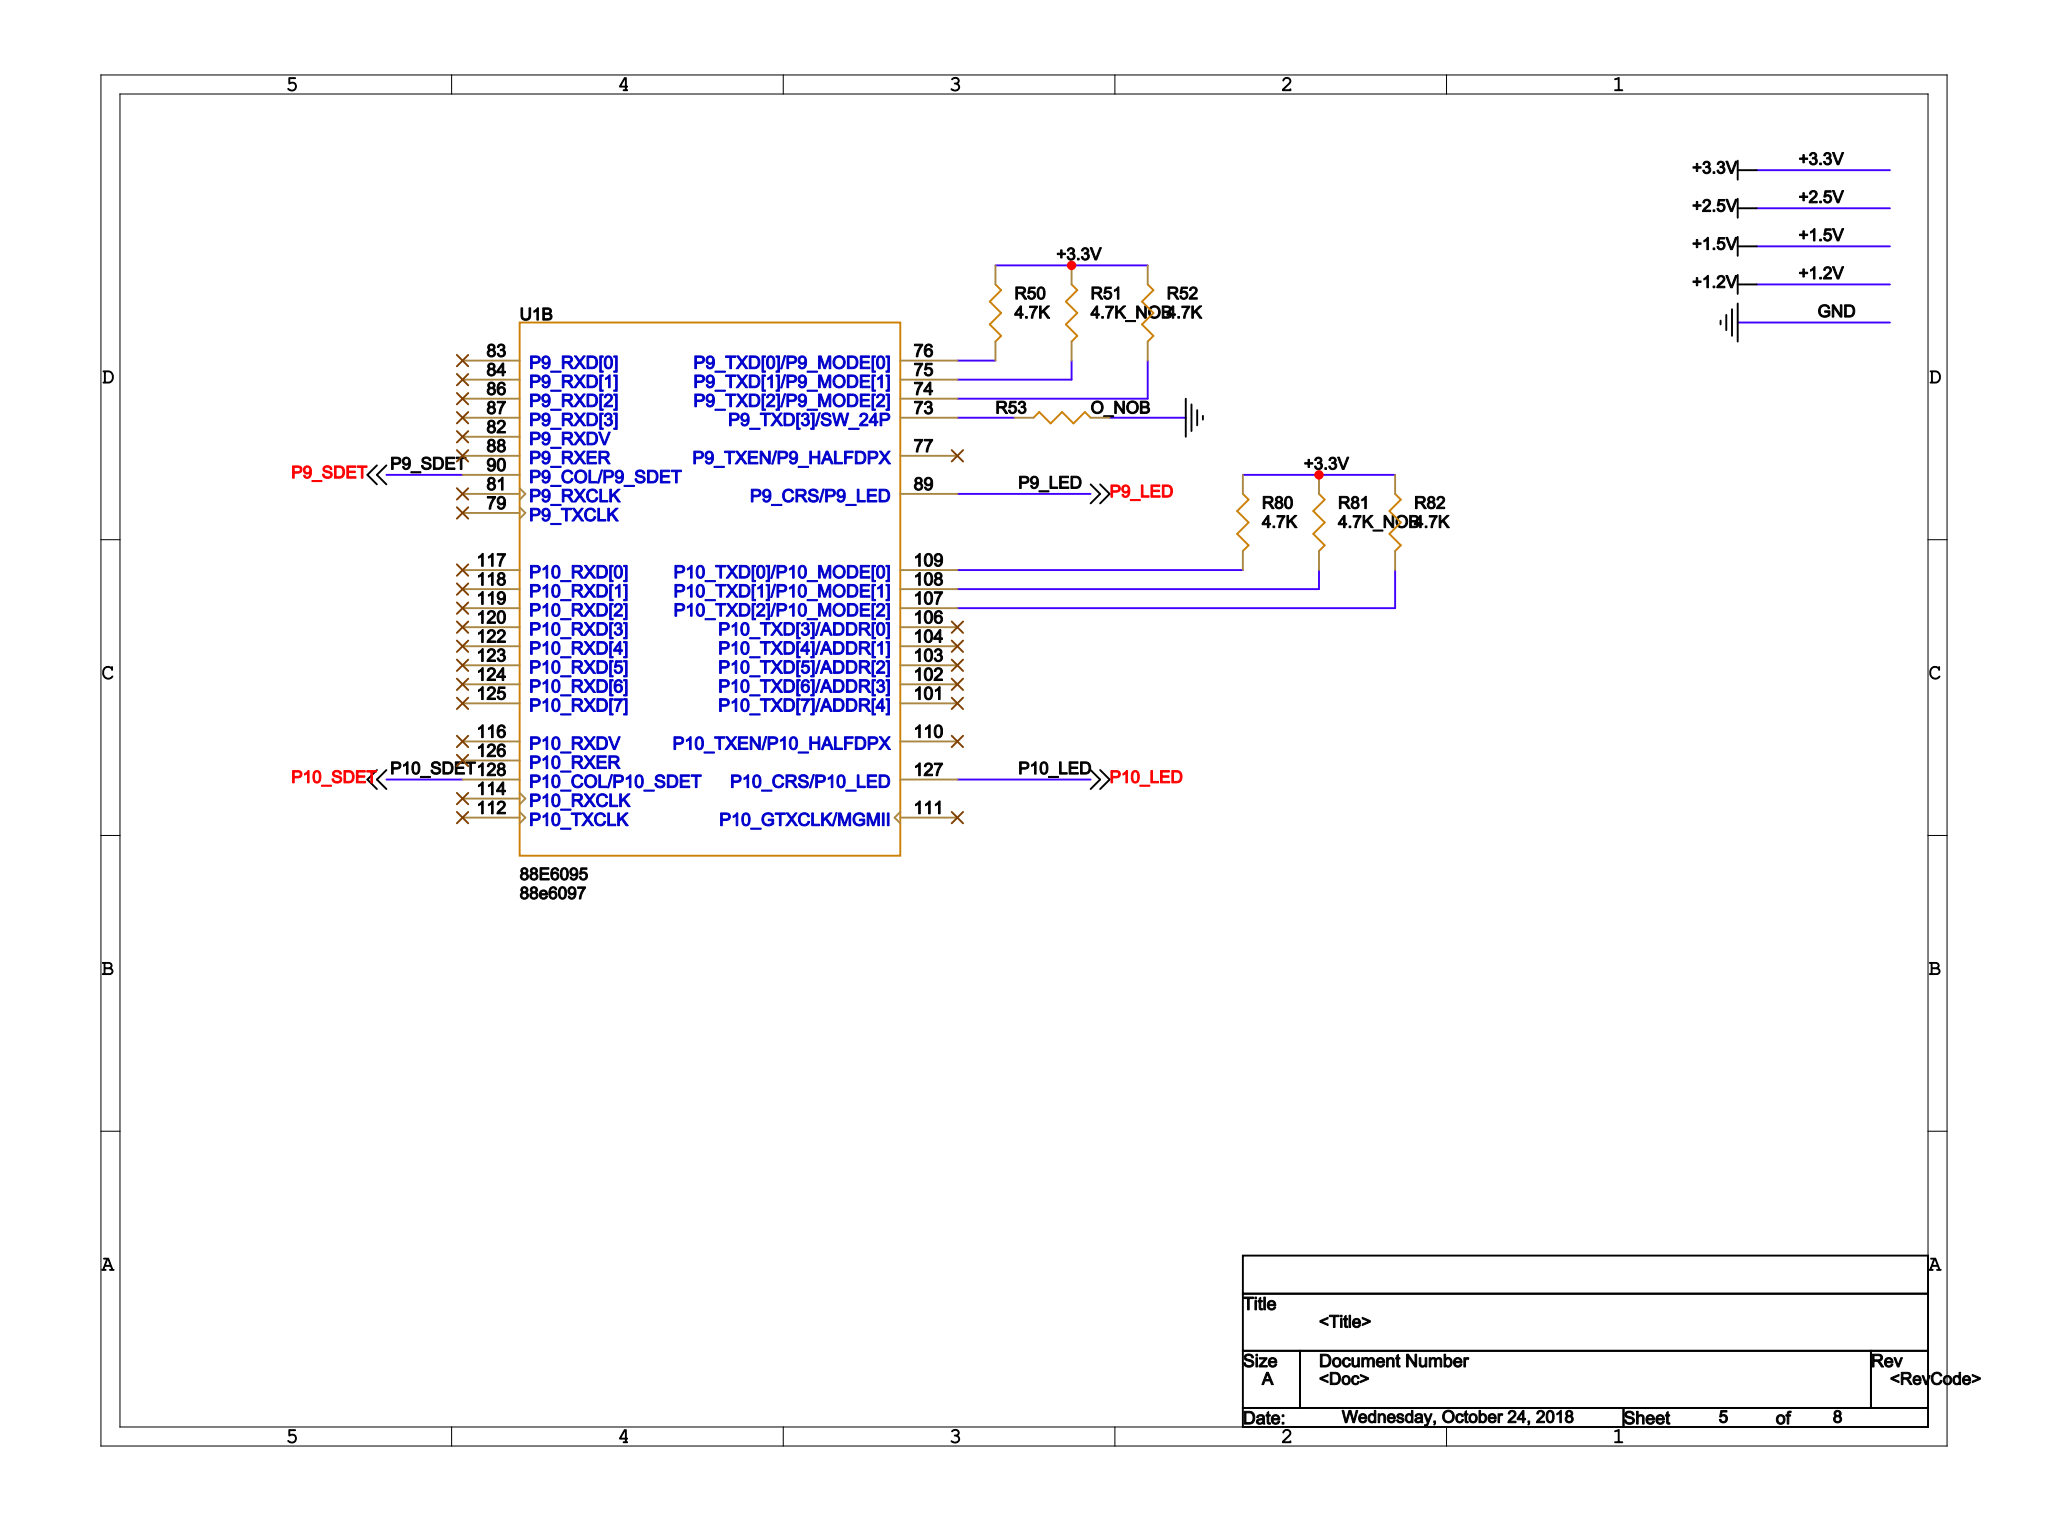Circuit board | Cadence Allegro | 219 parts | 174 nets | one sheet of the schematic
Parts on this sheet (reference | value | footprint):
R50 | 4.7K | SR0603
R51 | 4.7K_NOB | SR0603
R52 | 4.7K | SR0603
R53 | O_NOB | SR0603
R80 | 4.7K | SR0603
R81 | 4.7K_NOB | SR0603
R82 | 4.7K | SR0603
U1 | 88E6095 | 88E6097
Nets of these parts (net: part-pin ...):
GND: R53-2
P10_SDET: U1-128
P10_LED: U1-127
N1409589: R80-2 U1-109
N1409593: R81-2 U1-108
N1409597: R82-2 U1-107
P9_SDET: U1-90
P9_LED: U1-89
N1342715: R50-2 U1-76
N1342719: R51-2 U1-75
N1342726: R52-2 U1-74
N1342906: R53-1 U1-73
+1.2V: U1-3 U1-8
+3.3V: R50-1 R51-1 R52-1 R80-1 R81-1 R82-1